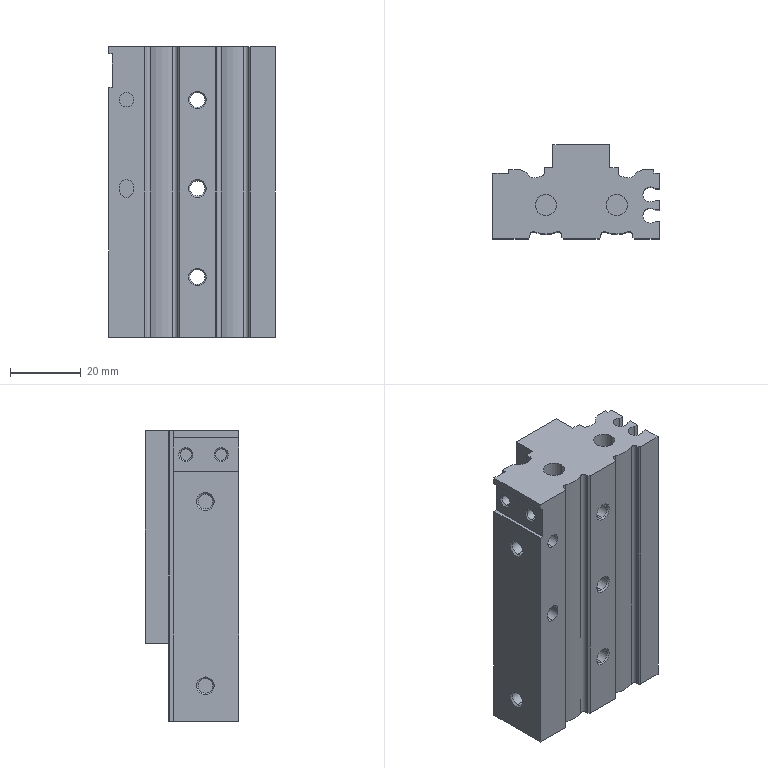Part | SolidWorks | features BaseBody 1 | 1 solid | 145 faces | box 47 x 26.5 x 82 mm | volume 60945 mm3 | plane 62 | cylinder 61 | cone 22 | commonest cylinder face diameters 3.242 x12 4.2 x10 4 x7 2 x6 4.134 x4 6 x4